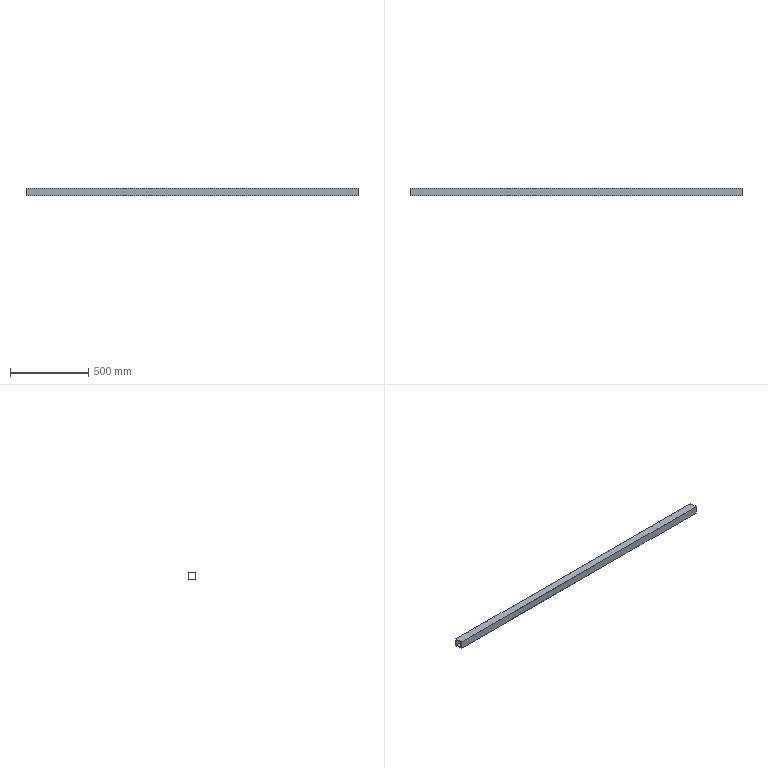Part | NX | features solid 2 | 1 solid | 10 faces | box 2120 x 50 x 50 mm | volume 1908000 mm3 | plane 10
STEP:
#1=CARTESIAN_POINT('',(-1060.,45.,1290.));
#2=VERTEX_POINT('',#1);
#3=CARTESIAN_POINT('',(-1060.,45.,1250.));
#4=VERTEX_POINT('',#3);
#5=CARTESIAN_POINT('',(-1060.,45.,1290.));
#6=DIRECTION('',(0.,0.,-1.));
#7=VECTOR('',#6,1000.);
#8=LINE('',#5,#7);
#9=EDGE_CURVE('',#2,#4,#8,.T.);
#10=ORIENTED_EDGE('',*,*,#9,.F.);
#11=CARTESIAN_POINT('',(-1060.,5.,1290.));
#12=VERTEX_POINT('',#11);
#13=CARTESIAN_POINT('',(-1060.,5.,1290.));
#14=DIRECTION('',(0.,1.,0.));
#15=VECTOR('',#14,1000.);
#16=LINE('',#13,#15);
#17=EDGE_CURVE('',#12,#2,#16,.T.);
#18=ORIENTED_EDGE('',*,*,#17,.F.);
#19=CARTESIAN_POINT('',(-1060.,5.,1250.));
#20=VERTEX_POINT('',#19);
#21=CARTESIAN_POINT('',(-1060.,5.,1250.));
#22=DIRECTION('',(0.,0.,1.));
#23=VECTOR('',#22,1000.);
#24=LINE('',#21,#23);
#25=EDGE_CURVE('',#20,#12,#24,.T.);
#26=ORIENTED_EDGE('',*,*,#25,.F.);
#27=CARTESIAN_POINT('',(-1060.,45.,1250.));
#28=DIRECTION('',(0.,-1.,0.));
#29=VECTOR('',#28,1000.);
#30=LINE('',#27,#29);
#31=EDGE_CURVE('',#4,#20,#30,.T.);
#32=ORIENTED_EDGE('',*,*,#31,.F.);
#33=EDGE_LOOP('',(#10,#18,#26,#32));
#34=FACE_BOUND('',#33,.T.);
#35=CARTESIAN_POINT('',(-1060.,0.,1245.));
#36=VERTEX_POINT('',#35);
#37=CARTESIAN_POINT('',(-1060.,0.,1295.));
#38=VERTEX_POINT('',#37);
#39=CARTESIAN_POINT('',(-1060.,0.,1245.));
#40=DIRECTION('',(0.,0.,1.));
#41=VECTOR('',#40,1000.);
#42=LINE('',#39,#41);
#43=EDGE_CURVE('',#36,#38,#42,.T.);
#44=ORIENTED_EDGE('',*,*,#43,.T.);
#45=CARTESIAN_POINT('',(-1060.,50.,1295.));
#46=VERTEX_POINT('',#45);
#47=CARTESIAN_POINT('',(-1060.,-2101.162,1295.));
#48=DIRECTION('',(0.,1.,0.));
#49=VECTOR('',#48,1000.);
#50=LINE('',#47,#49);
#51=EDGE_CURVE('',#38,#46,#50,.T.);
#52=ORIENTED_EDGE('',*,*,#51,.T.);
#53=CARTESIAN_POINT('',(-1060.,50.,1245.));
#54=VERTEX_POINT('',#53);
#55=CARTESIAN_POINT('',(-1060.,50.,1245.));
#56=DIRECTION('',(0.,0.,1.));
#57=VECTOR('',#56,1000.);
#58=LINE('',#55,#57);
#59=EDGE_CURVE('',#54,#46,#58,.T.);
#60=ORIENTED_EDGE('',*,*,#59,.F.);
#61=CARTESIAN_POINT('',(-1060.,-2101.162,1245.));
#62=DIRECTION('',(0.,1.,0.));
#63=VECTOR('',#62,1000.);
#64=LINE('',#61,#63);
#65=EDGE_CURVE('',#36,#54,#64,.T.);
#66=ORIENTED_EDGE('',*,*,#65,.F.);
#67=EDGE_LOOP('',(#44,#52,#60,#66));
#68=FACE_BOUND('',#67,.T.);
#69=CARTESIAN_POINT('',(-1060.,-2101.162,1245.));
#70=DIRECTION('',(-1.,0.,0.));
#71=DIRECTION('',(0.,0.,1.));
#72=AXIS2_PLACEMENT_3D('',#69,#70,#71);
#73=PLANE('',#72);
#74=ADVANCED_FACE('',(#34,#68),#73,.T.);
#75=CARTESIAN_POINT('',(1060.,5.,1290.));
#76=VERTEX_POINT('',#75);
#77=CARTESIAN_POINT('',(1060.,5.,1250.));
#78=VERTEX_POINT('',#77);
#79=CARTESIAN_POINT('',(1060.,5.,1250.));
#80=DIRECTION('',(0.,0.,-1.));
#81=VECTOR('',#80,1000.);
#82=LINE('',#79,#81);
#83=EDGE_CURVE('',#76,#78,#82,.T.);
#84=ORIENTED_EDGE('',*,*,#83,.F.);
#85=CARTESIAN_POINT('',(1060.,45.,1290.));
#86=VERTEX_POINT('',#85);
#87=CARTESIAN_POINT('',(1060.,5.,1290.));
#88=DIRECTION('',(0.,-1.,0.));
#89=VECTOR('',#88,1000.);
#90=LINE('',#87,#89);
#91=EDGE_CURVE('',#86,#76,#90,.T.);
#92=ORIENTED_EDGE('',*,*,#91,.F.);
#93=CARTESIAN_POINT('',(1060.,45.,1250.));
#94=VERTEX_POINT('',#93);
#95=CARTESIAN_POINT('',(1060.,45.,1290.));
#96=DIRECTION('',(0.,0.,1.));
#97=VECTOR('',#96,1000.);
#98=LINE('',#95,#97);
#99=EDGE_CURVE('',#94,#86,#98,.T.);
#100=ORIENTED_EDGE('',*,*,#99,.F.);
#101=CARTESIAN_POINT('',(1060.,45.,1250.));
#102=DIRECTION('',(0.,1.,0.));
#103=VECTOR('',#102,1000.);
#104=LINE('',#101,#103);
#105=EDGE_CURVE('',#78,#94,#104,.T.);
#106=ORIENTED_EDGE('',*,*,#105,.F.);
#107=EDGE_LOOP('',(#84,#92,#100,#106));
#108=FACE_BOUND('',#107,.T.);
#109=CARTESIAN_POINT('',(1060.,0.,1295.));
#110=VERTEX_POINT('',#109);
#111=CARTESIAN_POINT('',(1060.,0.,1245.));
#112=VERTEX_POINT('',#111);
#113=CARTESIAN_POINT('',(1060.,0.,1245.));
#114=DIRECTION('',(0.,0.,-1.));
#115=VECTOR('',#114,1000.);
#116=LINE('',#113,#115);
#117=EDGE_CURVE('',#110,#112,#116,.T.);
#118=ORIENTED_EDGE('',*,*,#117,.T.);
#119=CARTESIAN_POINT('',(1060.,50.,1245.));
#120=VERTEX_POINT('',#119);
#121=CARTESIAN_POINT('',(1060.,-2151.136,1245.));
#122=DIRECTION('',(0.,1.,0.));
#123=VECTOR('',#122,1000.);
#124=LINE('',#121,#123);
#125=EDGE_CURVE('',#112,#120,#124,.T.);
#126=ORIENTED_EDGE('',*,*,#125,.T.);
#127=CARTESIAN_POINT('',(1060.,50.,1295.));
#128=VERTEX_POINT('',#127);
#129=CARTESIAN_POINT('',(1060.,50.,1295.));
#130=DIRECTION('',(0.,0.,-1.));
#131=VECTOR('',#130,1000.);
#132=LINE('',#129,#131);
#133=EDGE_CURVE('',#128,#120,#132,.T.);
#134=ORIENTED_EDGE('',*,*,#133,.F.);
#135=CARTESIAN_POINT('',(1060.,-2151.136,1295.));
#136=DIRECTION('',(0.,1.,0.));
#137=VECTOR('',#136,1000.);
#138=LINE('',#135,#137);
#139=EDGE_CURVE('',#110,#128,#138,.T.);
#140=ORIENTED_EDGE('',*,*,#139,.F.);
#141=EDGE_LOOP('',(#118,#126,#134,#140));
#142=FACE_BOUND('',#141,.T.);
#143=CARTESIAN_POINT('',(1060.,-2151.136,1295.));
#144=DIRECTION('',(1.,0.,0.));
#145=DIRECTION('',(0.,-1.,0.));
#146=AXIS2_PLACEMENT_3D('',#143,#144,#145);
#147=PLANE('',#146);
#148=ADVANCED_FACE('',(#108,#142),#147,.T.);
#149=CARTESIAN_POINT('',(1110.,5.,1290.));
#150=DIRECTION('',(-1.,0.,0.));
#151=VECTOR('',#150,1000.);
#152=LINE('',#149,#151);
#153=EDGE_CURVE('',#76,#12,#152,.T.);
#154=ORIENTED_EDGE('',*,*,#153,.T.);
#155=ORIENTED_EDGE('',*,*,#17,.T.);
#156=CARTESIAN_POINT('',(-1090.,45.,1290.));
#157=DIRECTION('',(1.,0.,0.));
#158=VECTOR('',#157,1000.);
#159=LINE('',#156,#158);
#160=EDGE_CURVE('',#2,#86,#159,.T.);
#161=ORIENTED_EDGE('',*,*,#160,.T.);
#162=ORIENTED_EDGE('',*,*,#91,.T.);
#163=EDGE_LOOP('',(#154,#155,#161,#162));
#164=FACE_BOUND('',#163,.T.);
#165=CARTESIAN_POINT('',(1110.,5.,1290.));
#166=DIRECTION('',(0.,0.,-1.));
#167=DIRECTION('',(-1.,0.,0.));
#168=AXIS2_PLACEMENT_3D('',#165,#166,#167);
#169=PLANE('',#168);
#170=ADVANCED_FACE('',(#164),#169,.T.);
#171=ORIENTED_EDGE('',*,*,#51,.F.);
#172=CARTESIAN_POINT('',(-1090.,0.,1295.));
#173=DIRECTION('',(-1.,0.,0.));
#174=VECTOR('',#173,1000.);
#175=LINE('',#172,#174);
#176=EDGE_CURVE('',#110,#38,#175,.T.);
#177=ORIENTED_EDGE('',*,*,#176,.F.);
#178=ORIENTED_EDGE('',*,*,#139,.T.);
#179=CARTESIAN_POINT('',(-1090.,50.,1295.));
#180=DIRECTION('',(1.,0.,0.));
#181=VECTOR('',#180,1000.);
#182=LINE('',#179,#181);
#183=EDGE_CURVE('',#46,#128,#182,.T.);
#184=ORIENTED_EDGE('',*,*,#183,.F.);
#185=EDGE_LOOP('',(#171,#177,#178,#184));
#186=FACE_BOUND('',#185,.T.);
#187=CARTESIAN_POINT('',(1110.,0.,1295.));
#188=DIRECTION('',(0.,0.,-1.));
#189=DIRECTION('',(-1.,0.,0.));
#190=AXIS2_PLACEMENT_3D('',#187,#188,#189);
#191=PLANE('',#190);
#192=ADVANCED_FACE('',(#186),#191,.F.);
#193=CARTESIAN_POINT('',(-1090.,5.,1250.));
#194=DIRECTION('',(-1.,0.,0.));
#195=VECTOR('',#194,1000.);
#196=LINE('',#193,#195);
#197=EDGE_CURVE('',#78,#20,#196,.T.);
#198=ORIENTED_EDGE('',*,*,#197,.T.);
#199=ORIENTED_EDGE('',*,*,#25,.T.);
#200=ORIENTED_EDGE('',*,*,#153,.F.);
#201=ORIENTED_EDGE('',*,*,#83,.T.);
#202=EDGE_LOOP('',(#198,#199,#200,#201));
#203=FACE_BOUND('',#202,.T.);
#204=CARTESIAN_POINT('',(1110.,5.,1250.));
#205=DIRECTION('',(0.,1.,0.));
#206=DIRECTION('',(1.,0.,0.));
#207=AXIS2_PLACEMENT_3D('',#204,#205,#206);
#208=PLANE('',#207);
#209=ADVANCED_FACE('',(#203),#208,.T.);
#210=ORIENTED_EDGE('',*,*,#160,.F.);
#211=ORIENTED_EDGE('',*,*,#9,.T.);
#212=CARTESIAN_POINT('',(-1090.,45.,1250.));
#213=DIRECTION('',(1.,0.,0.));
#214=VECTOR('',#213,1000.);
#215=LINE('',#212,#214);
#216=EDGE_CURVE('',#4,#94,#215,.T.);
#217=ORIENTED_EDGE('',*,*,#216,.T.);
#218=ORIENTED_EDGE('',*,*,#99,.T.);
#219=EDGE_LOOP('',(#210,#211,#217,#218));
#220=FACE_BOUND('',#219,.T.);
#221=CARTESIAN_POINT('',(-1090.,45.,1290.));
#222=DIRECTION('',(0.,-1.,0.));
#223=DIRECTION('',(-1.,0.,0.));
#224=AXIS2_PLACEMENT_3D('',#221,#222,#223);
#225=PLANE('',#224);
#226=ADVANCED_FACE('',(#220),#225,.T.);
#227=ORIENTED_EDGE('',*,*,#43,.F.);
#228=CARTESIAN_POINT('',(-1090.,0.,1245.));
#229=DIRECTION('',(-1.,0.,0.));
#230=VECTOR('',#229,1000.);
#231=LINE('',#228,#230);
#232=EDGE_CURVE('',#112,#36,#231,.T.);
#233=ORIENTED_EDGE('',*,*,#232,.F.);
#234=ORIENTED_EDGE('',*,*,#117,.F.);
#235=ORIENTED_EDGE('',*,*,#176,.T.);
#236=EDGE_LOOP('',(#227,#233,#234,#235));
#237=FACE_BOUND('',#236,.T.);
#238=CARTESIAN_POINT('',(-1090.,0.,1245.));
#239=DIRECTION('',(0.,1.,0.));
#240=DIRECTION('',(1.,0.,0.));
#241=AXIS2_PLACEMENT_3D('',#238,#239,#240);
#242=PLANE('',#241);
#243=ADVANCED_FACE('',(#237),#242,.F.);
#244=ORIENTED_EDGE('',*,*,#59,.T.);
#245=ORIENTED_EDGE('',*,*,#183,.T.);
#246=ORIENTED_EDGE('',*,*,#133,.T.);
#247=CARTESIAN_POINT('',(-1090.,50.,1245.));
#248=DIRECTION('',(1.,0.,0.));
#249=VECTOR('',#248,1000.);
#250=LINE('',#247,#249);
#251=EDGE_CURVE('',#54,#120,#250,.T.);
#252=ORIENTED_EDGE('',*,*,#251,.F.);
#253=EDGE_LOOP('',(#244,#245,#246,#252));
#254=FACE_BOUND('',#253,.T.);
#255=CARTESIAN_POINT('',(-1090.,50.,1295.));
#256=DIRECTION('',(0.,-1.,0.));
#257=DIRECTION('',(-1.,0.,0.));
#258=AXIS2_PLACEMENT_3D('',#255,#256,#257);
#259=PLANE('',#258);
#260=ADVANCED_FACE('',(#254),#259,.F.);
#261=ORIENTED_EDGE('',*,*,#216,.F.);
#262=ORIENTED_EDGE('',*,*,#31,.T.);
#263=ORIENTED_EDGE('',*,*,#197,.F.);
#264=ORIENTED_EDGE('',*,*,#105,.T.);
#265=EDGE_LOOP('',(#261,#262,#263,#264));
#266=FACE_BOUND('',#265,.T.);
#267=CARTESIAN_POINT('',(-1090.,45.,1250.));
#268=DIRECTION('',(0.,0.,1.));
#269=DIRECTION('',(0.,-1.,0.));
#270=AXIS2_PLACEMENT_3D('',#267,#268,#269);
#271=PLANE('',#270);
#272=ADVANCED_FACE('',(#266),#271,.T.);
#273=ORIENTED_EDGE('',*,*,#65,.T.);
#274=ORIENTED_EDGE('',*,*,#251,.T.);
#275=ORIENTED_EDGE('',*,*,#125,.F.);
#276=ORIENTED_EDGE('',*,*,#232,.T.);
#277=EDGE_LOOP('',(#273,#274,#275,#276));
#278=FACE_BOUND('',#277,.T.);
#279=CARTESIAN_POINT('',(-1090.,0.,1245.));
#280=DIRECTION('',(0.,0.,1.));
#281=DIRECTION('',(0.,-1.,0.));
#282=AXIS2_PLACEMENT_3D('',#279,#280,#281);
#283=PLANE('',#282);
#284=ADVANCED_FACE('',(#278),#283,.F.);
#285=CLOSED_SHELL('',(#74,#148,#170,#192,#209,#226,#243,#260,#272,#284));
#286=MANIFOLD_SOLID_BREP('',#285);
#287=(LENGTH_UNIT()NAMED_UNIT(*)SI_UNIT(.MILLI.,.METRE.));
#288=UNCERTAINTY_MEASURE_WITH_UNIT(LENGTH_MEASURE(0.00001),#287,'','');
#289=(NAMED_UNIT(*)PLANE_ANGLE_UNIT()SI_UNIT($,.RADIAN.));
#290=(NAMED_UNIT(*)SI_UNIT($,.STERADIAN.)SOLID_ANGLE_UNIT());
#291=(GEOMETRIC_REPRESENTATION_CONTEXT(3)GLOBAL_UNCERTAINTY_ASSIGNED_CONTEXT((#288))GLOBAL_UNIT_ASSIGNED_CONTEXT((#287,#289,#290))REPRESENTATION_CONTEXT('',''));
#292=ADVANCED_BREP_SHAPE_REPRESENTATION('',(#286),#291);